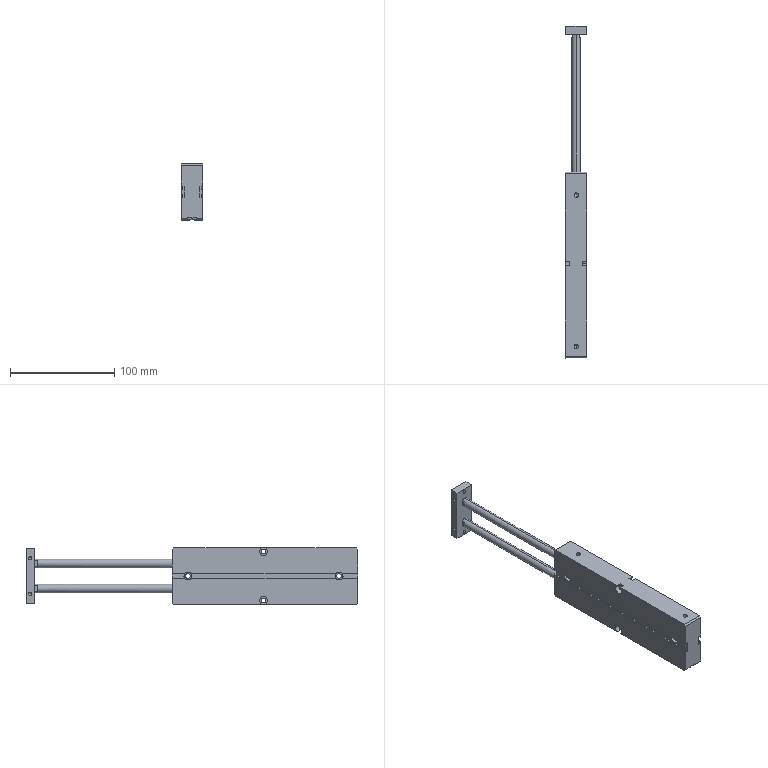Part | STEP file | TN-16×125-S Extend | 2 solids | 135 faces | box 21 x 318 x 54 mm | volume 212013 mm3 | plane 69 | cylinder 54 | cone 12 | commonest cylinder face diameters 7.5 x20 3.3 x12 8 x10 4.5 x8 4.2 x4